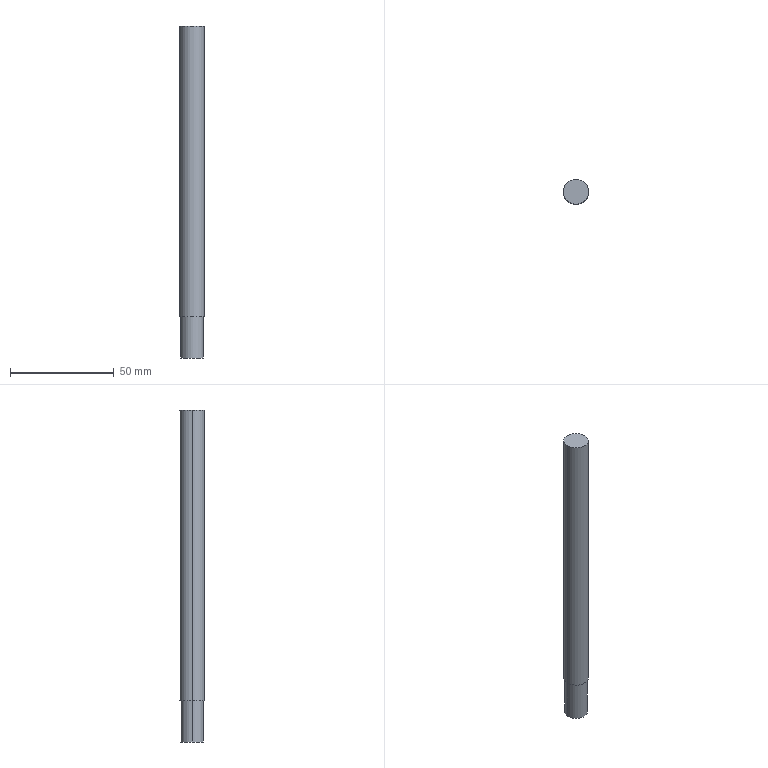Part | SolidWorks | features MirrorStock 1 | 1 solid | 7 faces | box 12 x 12 x 160 mm | volume 17734 mm3 | cylinder 4 | plane 3 | commonest cylinder face diameters 11 x2 12 x2
STEP:
#1=CARTESIAN_POINT('',(-5.5,0.,-60.));
#2=VERTEX_POINT('',#1);
#3=CARTESIAN_POINT('',(5.5,0.,-60.));
#4=VERTEX_POINT('',#3);
#5=CARTESIAN_POINT('',(0.,0.,-60.));
#6=DIRECTION('',(0.,0.,1.));
#7=DIRECTION('',(1.,0.,0.));
#8=AXIS2_PLACEMENT_3D('',#5,#6,#7);
#9=CIRCLE('',#8,5.5);
#10=EDGE_CURVE('',#2,#4,#9,.T.);
#11=ORIENTED_EDGE('',*,*,#10,.F.);
#12=CARTESIAN_POINT('',(-5.5,0.,-80.));
#13=VERTEX_POINT('',#12);
#14=CARTESIAN_POINT('',(-5.5,0.,-60.));
#15=DIRECTION('',(0.,0.,-1.));
#16=VECTOR('',#15,1000.);
#17=LINE('',#14,#16);
#18=EDGE_CURVE('',#2,#13,#17,.T.);
#19=ORIENTED_EDGE('',*,*,#18,.T.);
#20=CARTESIAN_POINT('',(5.5,0.,-80.));
#21=VERTEX_POINT('',#20);
#22=CARTESIAN_POINT('',(0.,0.,-80.));
#23=DIRECTION('',(0.,0.,1.));
#24=DIRECTION('',(1.,0.,0.));
#25=AXIS2_PLACEMENT_3D('',#22,#23,#24);
#26=CIRCLE('',#25,5.5);
#27=EDGE_CURVE('',#13,#21,#26,.T.);
#28=ORIENTED_EDGE('',*,*,#27,.T.);
#29=CARTESIAN_POINT('',(5.5,0.,-60.));
#30=DIRECTION('',(0.,0.,-1.));
#31=VECTOR('',#30,1000.);
#32=LINE('',#29,#31);
#33=EDGE_CURVE('',#4,#21,#32,.T.);
#34=ORIENTED_EDGE('',*,*,#33,.F.);
#35=EDGE_LOOP('',(#11,#19,#28,#34));
#36=FACE_OUTER_BOUND('',#35,.T.);
#37=CARTESIAN_POINT('',(0.,0.,-60.));
#38=DIRECTION('',(0.,0.,-1.));
#39=DIRECTION('',(1.,0.,0.));
#40=AXIS2_PLACEMENT_3D('',#37,#38,#39);
#41=CYLINDRICAL_SURFACE('',#40,5.5);
#42=ADVANCED_FACE('',(#36),#41,.T.);
#43=CARTESIAN_POINT('',(-6.,0.,-60.));
#44=VERTEX_POINT('',#43);
#45=CARTESIAN_POINT('',(6.,0.,-60.));
#46=VERTEX_POINT('',#45);
#47=CARTESIAN_POINT('',(0.,0.,-60.));
#48=DIRECTION('',(0.,0.,1.));
#49=DIRECTION('',(1.,0.,0.));
#50=AXIS2_PLACEMENT_3D('',#47,#48,#49);
#51=CIRCLE('',#50,6.);
#52=EDGE_CURVE('',#44,#46,#51,.T.);
#53=ORIENTED_EDGE('',*,*,#52,.T.);
#54=CARTESIAN_POINT('',(6.,0.,80.));
#55=VERTEX_POINT('',#54);
#56=CARTESIAN_POINT('',(6.,0.,-80.));
#57=DIRECTION('',(0.,0.,1.));
#58=VECTOR('',#57,1000.);
#59=LINE('',#56,#58);
#60=EDGE_CURVE('',#46,#55,#59,.T.);
#61=ORIENTED_EDGE('',*,*,#60,.T.);
#62=CARTESIAN_POINT('',(-6.,0.,80.));
#63=VERTEX_POINT('',#62);
#64=CARTESIAN_POINT('',(0.,0.,80.));
#65=DIRECTION('',(0.,0.,1.));
#66=DIRECTION('',(1.,0.,0.));
#67=AXIS2_PLACEMENT_3D('',#64,#65,#66);
#68=CIRCLE('',#67,6.);
#69=EDGE_CURVE('',#63,#55,#68,.T.);
#70=ORIENTED_EDGE('',*,*,#69,.F.);
#71=CARTESIAN_POINT('',(-6.,0.,-80.));
#72=DIRECTION('',(0.,0.,1.));
#73=VECTOR('',#72,1000.);
#74=LINE('',#71,#73);
#75=EDGE_CURVE('',#44,#63,#74,.T.);
#76=ORIENTED_EDGE('',*,*,#75,.F.);
#77=EDGE_LOOP('',(#53,#61,#70,#76));
#78=FACE_OUTER_BOUND('',#77,.T.);
#79=CARTESIAN_POINT('',(0.,0.,-80.));
#80=DIRECTION('',(0.,0.,1.));
#81=DIRECTION('',(-1.,0.,0.));
#82=AXIS2_PLACEMENT_3D('',#79,#80,#81);
#83=CYLINDRICAL_SURFACE('',#82,6.);
#84=ADVANCED_FACE('',(#78),#83,.T.);
#85=ORIENTED_EDGE('',*,*,#60,.F.);
#86=CARTESIAN_POINT('',(0.,0.,-60.));
#87=DIRECTION('',(0.,0.,1.));
#88=DIRECTION('',(1.,0.,0.));
#89=AXIS2_PLACEMENT_3D('',#86,#87,#88);
#90=CIRCLE('',#89,6.);
#91=EDGE_CURVE('',#46,#44,#90,.T.);
#92=ORIENTED_EDGE('',*,*,#91,.T.);
#93=ORIENTED_EDGE('',*,*,#75,.T.);
#94=CARTESIAN_POINT('',(0.,0.,80.));
#95=DIRECTION('',(0.,0.,1.));
#96=DIRECTION('',(1.,0.,0.));
#97=AXIS2_PLACEMENT_3D('',#94,#95,#96);
#98=CIRCLE('',#97,6.);
#99=EDGE_CURVE('',#55,#63,#98,.T.);
#100=ORIENTED_EDGE('',*,*,#99,.F.);
#101=EDGE_LOOP('',(#85,#92,#93,#100));
#102=FACE_OUTER_BOUND('',#101,.T.);
#103=CARTESIAN_POINT('',(0.,0.,-80.));
#104=DIRECTION('',(0.,0.,1.));
#105=DIRECTION('',(-1.,0.,0.));
#106=AXIS2_PLACEMENT_3D('',#103,#104,#105);
#107=CYLINDRICAL_SURFACE('',#106,6.);
#108=ADVANCED_FACE('',(#102),#107,.T.);
#109=ORIENTED_EDGE('',*,*,#69,.T.);
#110=ORIENTED_EDGE('',*,*,#99,.T.);
#111=EDGE_LOOP('',(#109,#110));
#112=FACE_OUTER_BOUND('',#111,.T.);
#113=CARTESIAN_POINT('',(0.,0.,80.));
#114=DIRECTION('',(0.,0.,-1.));
#115=DIRECTION('',(1.,0.,0.));
#116=AXIS2_PLACEMENT_3D('',#113,#114,#115);
#117=PLANE('',#116);
#118=ADVANCED_FACE('',(#112),#117,.F.);
#119=CARTESIAN_POINT('',(0.,0.,-60.));
#120=DIRECTION('',(0.,0.,1.));
#121=DIRECTION('',(1.,0.,0.));
#122=AXIS2_PLACEMENT_3D('',#119,#120,#121);
#123=CIRCLE('',#122,5.5);
#124=EDGE_CURVE('',#4,#2,#123,.T.);
#125=ORIENTED_EDGE('',*,*,#124,.T.);
#126=ORIENTED_EDGE('',*,*,#10,.T.);
#127=EDGE_LOOP('',(#125,#126));
#128=FACE_BOUND('',#127,.T.);
#129=ORIENTED_EDGE('',*,*,#52,.F.);
#130=ORIENTED_EDGE('',*,*,#91,.F.);
#131=EDGE_LOOP('',(#129,#130));
#132=FACE_OUTER_BOUND('',#131,.T.);
#133=CARTESIAN_POINT('',(0.,0.,-60.));
#134=DIRECTION('',(0.,0.,-1.));
#135=DIRECTION('',(1.,0.,0.));
#136=AXIS2_PLACEMENT_3D('',#133,#134,#135);
#137=PLANE('',#136);
#138=ADVANCED_FACE('',(#128,#132),#137,.T.);
#139=ORIENTED_EDGE('',*,*,#18,.F.);
#140=ORIENTED_EDGE('',*,*,#124,.F.);
#141=ORIENTED_EDGE('',*,*,#33,.T.);
#142=CARTESIAN_POINT('',(0.,0.,-80.));
#143=DIRECTION('',(0.,0.,1.));
#144=DIRECTION('',(1.,0.,0.));
#145=AXIS2_PLACEMENT_3D('',#142,#143,#144);
#146=CIRCLE('',#145,5.5);
#147=EDGE_CURVE('',#21,#13,#146,.T.);
#148=ORIENTED_EDGE('',*,*,#147,.T.);
#149=EDGE_LOOP('',(#139,#140,#141,#148));
#150=FACE_OUTER_BOUND('',#149,.T.);
#151=CARTESIAN_POINT('',(0.,0.,-60.));
#152=DIRECTION('',(0.,0.,-1.));
#153=DIRECTION('',(1.,0.,0.));
#154=AXIS2_PLACEMENT_3D('',#151,#152,#153);
#155=CYLINDRICAL_SURFACE('',#154,5.5);
#156=ADVANCED_FACE('',(#150),#155,.T.);
#157=ORIENTED_EDGE('',*,*,#147,.F.);
#158=ORIENTED_EDGE('',*,*,#27,.F.);
#159=EDGE_LOOP('',(#157,#158));
#160=FACE_OUTER_BOUND('',#159,.T.);
#161=CARTESIAN_POINT('',(0.,0.,-80.));
#162=DIRECTION('',(0.,0.,-1.));
#163=DIRECTION('',(1.,0.,0.));
#164=AXIS2_PLACEMENT_3D('',#161,#162,#163);
#165=PLANE('',#164);
#166=ADVANCED_FACE('',(#160),#165,.T.);
#167=CLOSED_SHELL('',(#42,#84,#108,#118,#138,#156,#166));
#168=MANIFOLD_SOLID_BREP('',#167);
#169=CARTESIAN_POINT('',(0.,0.,0.));
#170=DIRECTION('',(0.,0.,1.));
#171=DIRECTION('',(1.,0.,0.));
#172=AXIS2_PLACEMENT_3D('',#169,#170,#171);
#173=(LENGTH_UNIT()NAMED_UNIT(*)SI_UNIT(.MILLI.,.METRE.));
#174=UNCERTAINTY_MEASURE_WITH_UNIT(LENGTH_MEASURE(0.00001),#173,'','');
#175=(NAMED_UNIT(*)PLANE_ANGLE_UNIT()SI_UNIT($,.RADIAN.));
#176=(NAMED_UNIT(*)SI_UNIT($,.STERADIAN.)SOLID_ANGLE_UNIT());
#177=(GEOMETRIC_REPRESENTATION_CONTEXT(3)GLOBAL_UNCERTAINTY_ASSIGNED_CONTEXT((#174))GLOBAL_UNIT_ASSIGNED_CONTEXT((#173,#175,#176))REPRESENTATION_CONTEXT('',''));
#178=ADVANCED_BREP_SHAPE_REPRESENTATION('',(#168,#172),#177);